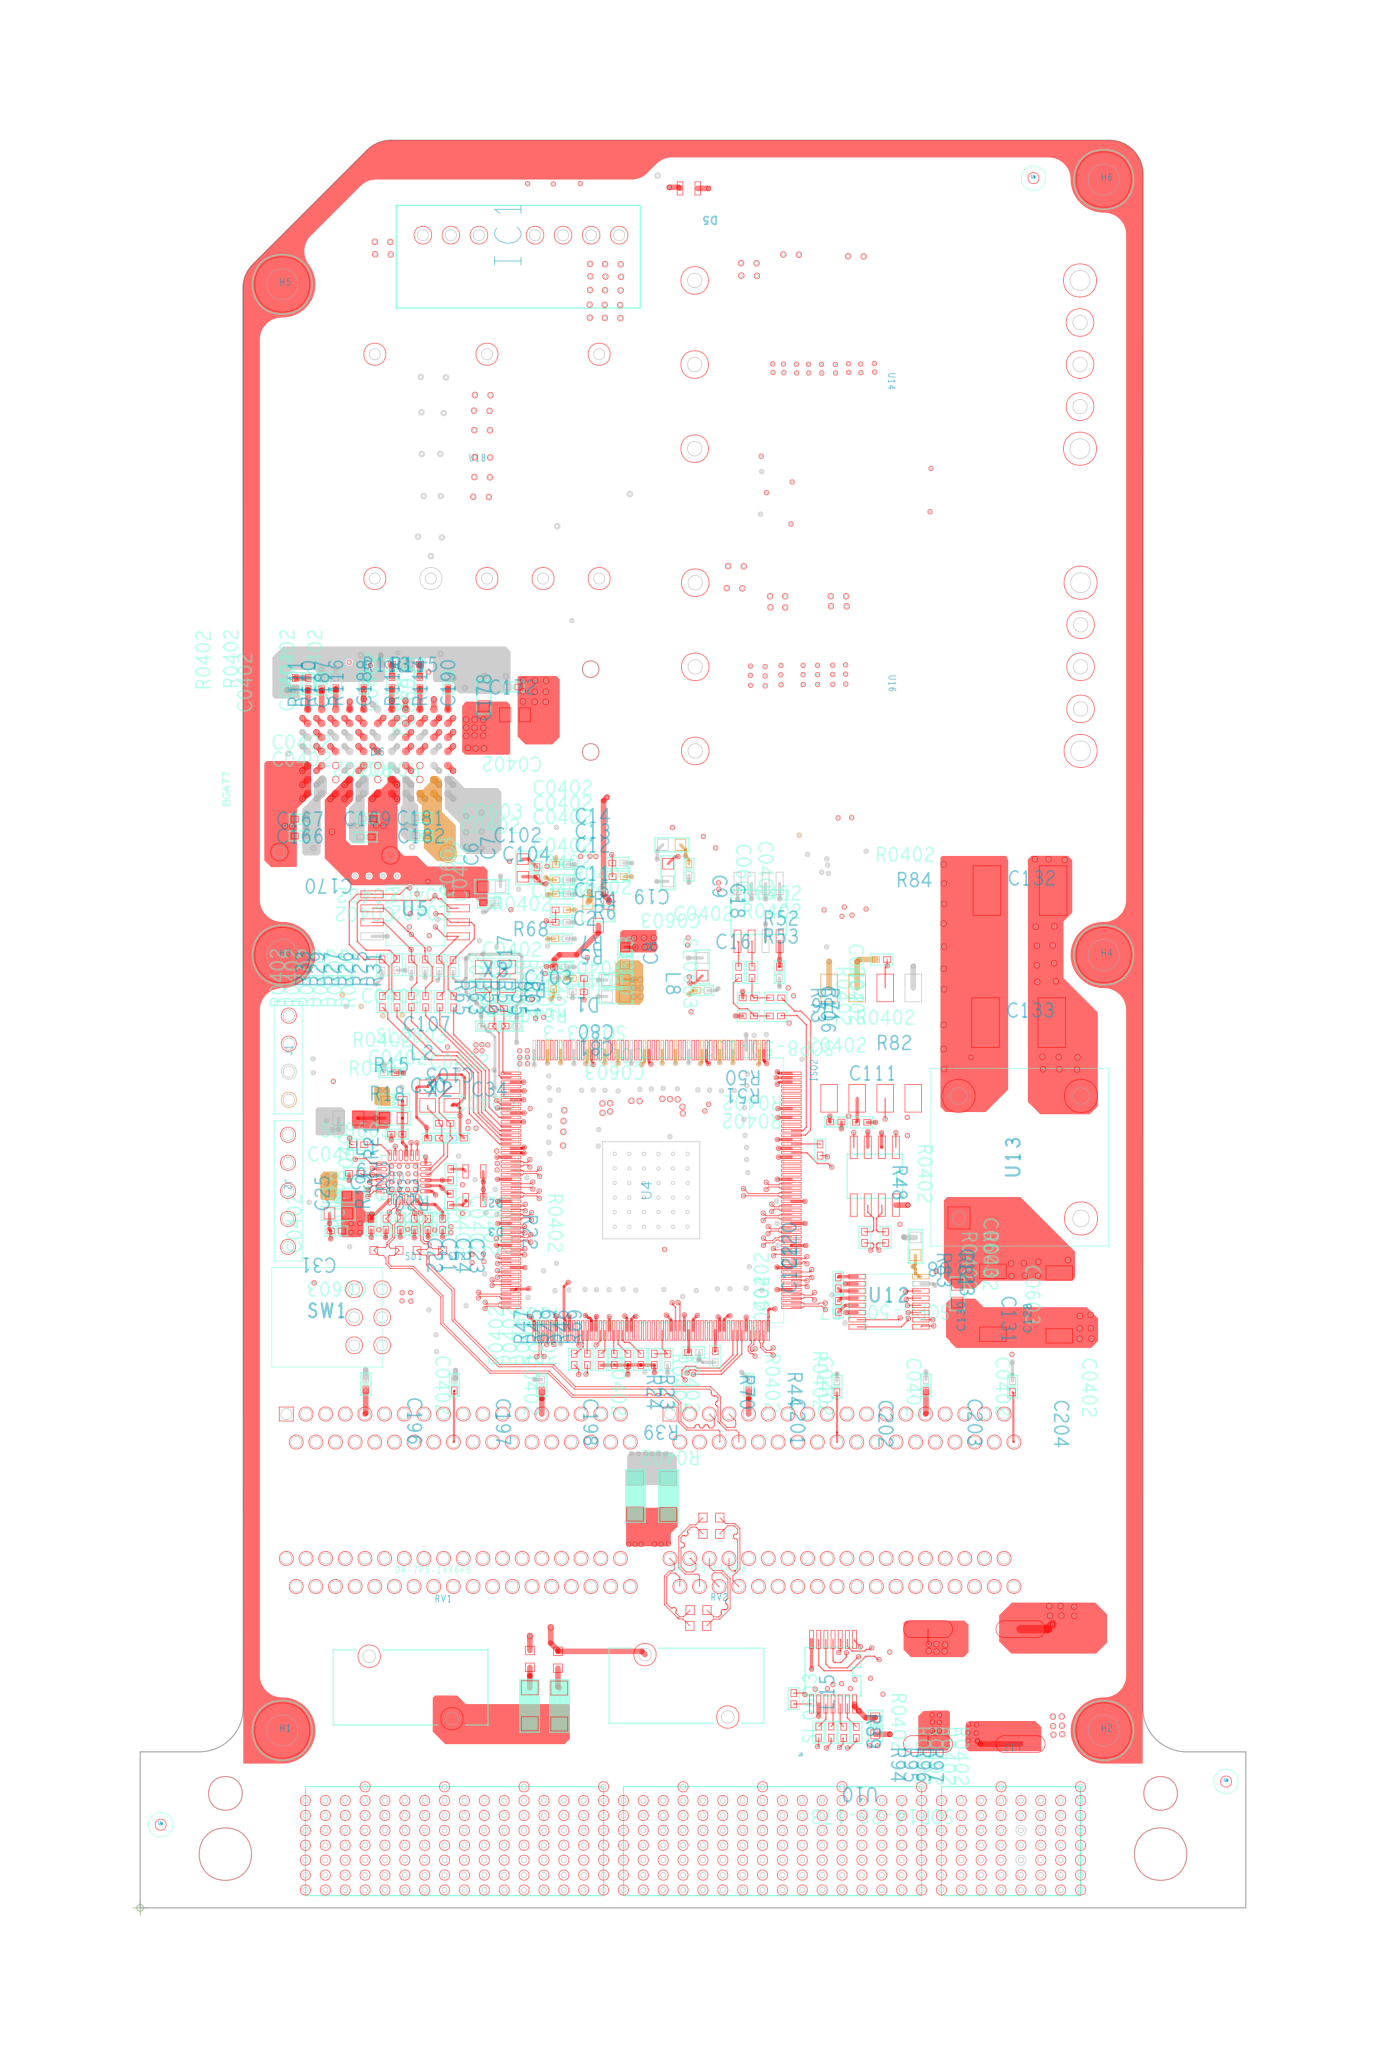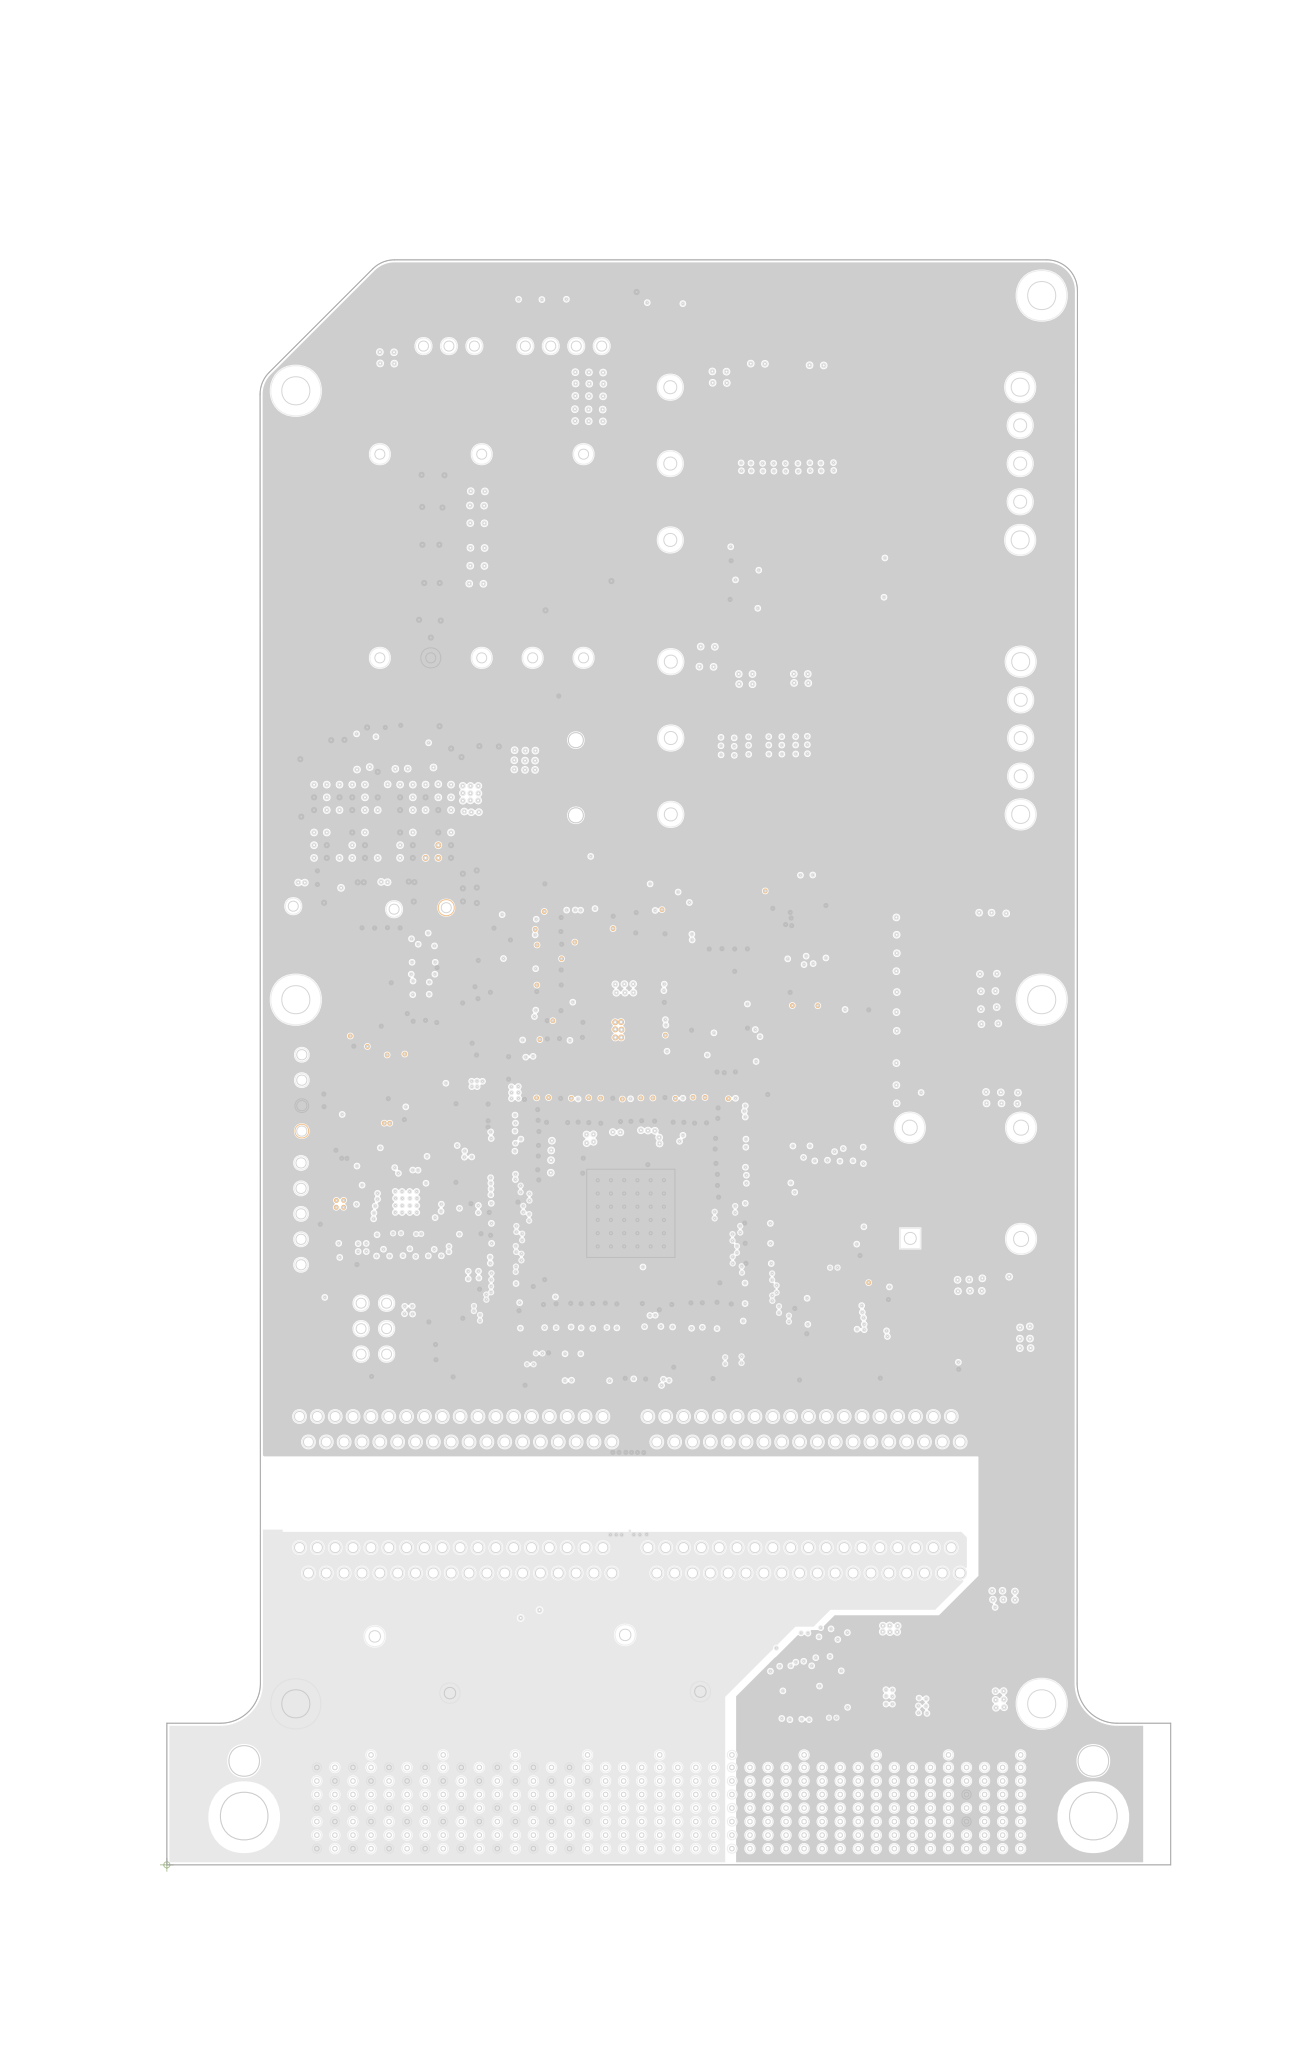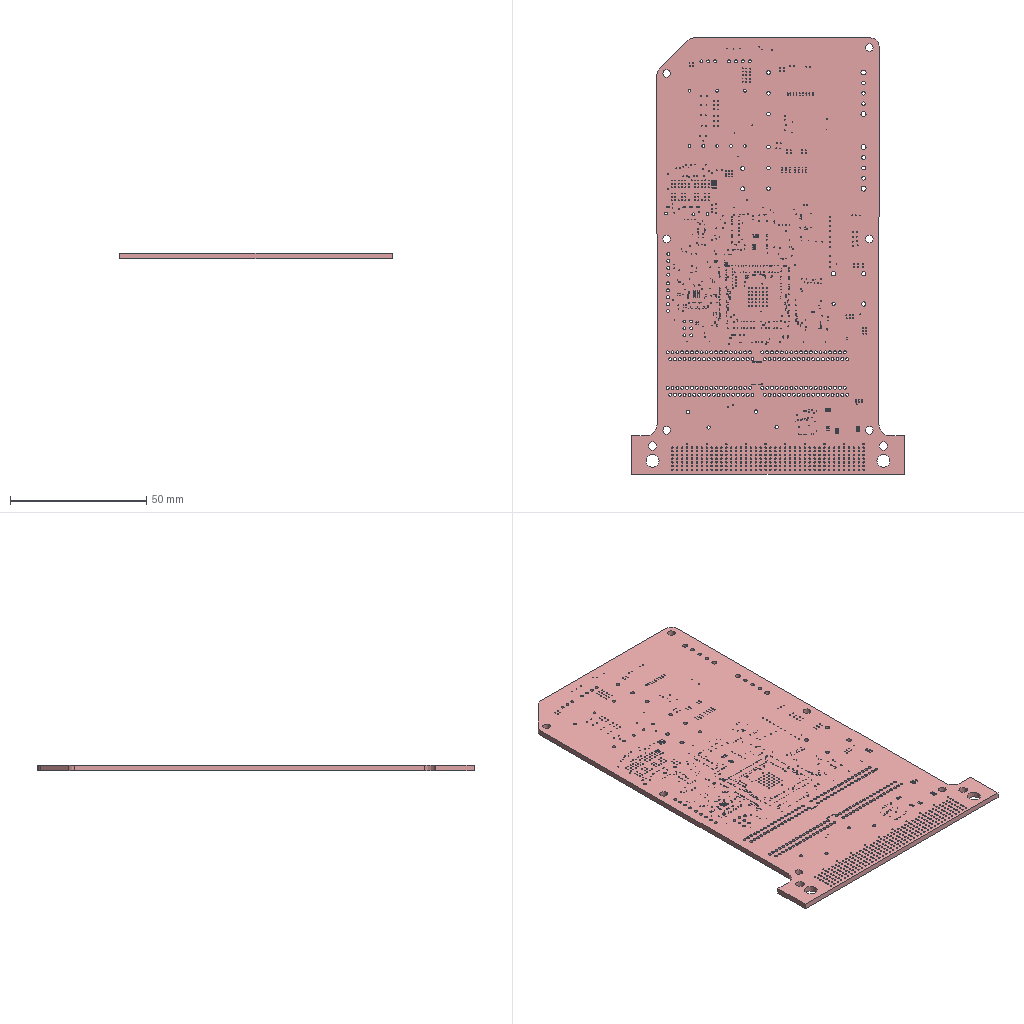Circuit board layout | Cadence Allegro | box 100.1 x 160.1 x 2.1 mm
Layer stack:
# Cadence Allegro layer stack of  (unit mm; from the constraint file cross-section; dielectric type: 0 not recorded (Allegro does not mark core vs prepreg), 3 surface material)
index,name,kind,layer,copper_thickness_mm,dielectric_type,dielectric_thickness_mm,dielectric_material,dielectric_constant
0,Top Surface,other,,,,,,
1,TOP,copper,TOP,0.0305,,,,
2,Dielectric1,dielectric,,,0,0.2032,FR-4,4.5
3,GND2,copper,GND2,0.0305,,,,
4,Dielectric2,dielectric,,,0,0.2032,FR-4,4.5
5,SIG3,copper,SIG3,0.0305,,,,
6,Dielectric3,dielectric,,,0,0.2032,FR-4,4.5
7,POWER4,copper,POWER4,0.0305,,,,
8,Dielectric4,dielectric,,,0,0.2032,FR-4,4.5
9,POWER5,copper,POWER5,0.0305,,,,
10,Dielectric5,dielectric,,,0,0.2032,FR-4,4.5
11,POWER6,copper,POWER6,0.0305,,,,
12,Dielectric6,dielectric,,,0,0.2032,FR-4,4.5
13,GND7,copper,GND7,0.0305,,,,
14,Dielectric7,dielectric,,,0,0.2032,FR-4,4.5
15,SIG8,copper,SIG8,0.0305,,,,
16,Dielectric8,dielectric,,,0,0.2032,FR-4,4.5
17,GND9,copper,GND9,0.0305,,,,
18,Dielectric9,dielectric,,,0,0.2032,FR-4,4.5
19,BOTTOM,copper,BOTTOM,0.0305,,,,
20,Bottom Surface,other,,,,,,
# drill layer pairs: low layer,high layer
drill_pair,TOP,BOTTOM
Part placement:
REFDES,COMP_VALUE,SYM_NAME,SYM_X,SYM_Y,SYM_ROTATE,SYM_MIRROR
BT1,CR1220,CR1220,1606.230,4275.930,270.000,YES
C1,2pF,SC0402,1221.830,3337.342,90.000,YES
C2,0.1uF/16V,SC0402,1496.000,3355.000,0.000,NO
C3,2pF,SC0402,1222.830,3247.342,270.000,YES
C4,20pF,SC0402,1246.470,3532.310,270.000,YES
C5,20pF,SC0402,1246.470,3447.310,90.000,YES
C6,1uF/50V,SC0603,1364.028,3708.722,90.000,NO
C7,0.1uF/16V,SC0402,1414.460,3690.992,90.000,NO
C8,2.2uF,SC0603,2004.278,3356.092,90.000,NO
C9,2.2uF,SC0603,1882.000,3692.000,270.000,NO
C10,0.1uF/16V,SC0402,663.890,2861.622,270.000,YES
C11,0.1uF/16V,SC0402,1501.000,3515.000,0.000,NO
C12,0.1uF/16V,SC0402,1502.000,3616.000,0.000,NO
C13,0.1uF/16V,SC0402,1502.000,3666.000,0.000,NO
C14,0.1uF/16V,SC0402,1502.000,3721.000,0.000,NO
C15,0.1uF/16V,SC0402,1499.000,3456.000,0.000,NO
C16,0.1uF/16V,SC0402,2003.884,3271.776,0.000,NO
C17,0.1uF/16V,SC0402,1474.000,3296.000,90.000,NO
C18,0.1uF/16V,SC0402,1956.210,3702.418,270.000,NO
C19,10uF/6.3V,SC0603,1895.000,3791.000,180.000,NO
C20,0.1uF/16V,SC0402,757.158,3235.510,90.000,YES
C21,10pF/16V,SC0402,927.190,2437.606,270.000,NO
C22,10pF/16V,SC0402,876.098,2438.000,270.000,NO
C23,10pF/16V,SC0402,1025.920,2437.424,270.000,NO
C24,10pF/16V,SC0402,977.252,2437.818,270.000,NO
C25,0.1uF/16V,SC0402,823.460,2437.284,90.000,NO
C26,0.1uF/16V,SC0402,1022.720,2735.994,90.000,YES
C27,0.1uF/16V,SC0402,1061.720,2735.994,90.000,YES
C28,0.1uF/16V,SC0402,1128.810,2502.688,0.000,YES
C29,10uF/6.3V,SC0603,903.442,2816.312,180.000,NO
C30,0.1uF/16V,SC0402,914.868,2758.788,0.000,NO
C31,10uF/6.3V,SC0603,706.442,2476.684,180.000,NO
C32,0.1uF/16V,SC0402,698.956,2414.038,0.000,NO
C33,20pF,SC0402,1046.034,2745.002,180.000,NO
C34,20pF,SC0402,1134.034,2745.002,0.000,NO
C35,10uF/6.3V,SC0603,1122.900,2178.426,90.000,YES
C36,0.1uF/16V,SC0402,2240.284,2157.150,270.000,YES
C37,0.1uF/16V,SC0402,2224.918,2285.988,0.000,YES
C38,0.1uF/16V,SC0402,2215.068,2622.464,0.000,YES
C39,0.1uF/16V,SC0402,1531.000,2158.000,270.000,YES
C40,0.1uF/16V,SC0402,2326.176,2441.224,0.000,YES
C41,0.1uF/16V,SC0402,1323.446,2603.158,180.000,YES
C42,0.1uF/16V,SC0402,1303.352,2455.408,270.000,YES
C43,0.1uF/16V,SC0402,1418.794,2294.656,180.000,YES
C44,0.1uF/16V,SC0402,1407.762,2156.362,270.000,YES
C45,0.1uF/16V,SC0402,2160.302,2161.484,270.000,YES
C46,0.1uF/16V,SC0402,1214.308,2620.888,0.000,YES
C47,0.1uF/16V,SC0402,2323.812,2520.812,0.000,YES
C48,0.1uF/16V,SC0402,2213.886,2667.380,0.000,YES
C49,0.1uF/16V,SC0402,2226.100,2234.374,0.000,YES
C50,10uF/6.3V,SC0603,1203.276,2680.776,0.000,YES
C51,0.1uF/16V,SC0402,1304.140,2542.482,270.000,YES
C52,0.1uF/16V,SC0402,1418.794,2231.222,180.000,YES
C53,0.1uF/16V,SC0402,1479.000,2157.000,270.000,YES
C54,10uF/6.3V,SC0603,1279.712,2956.182,0.000,YES
C55,0.1uF/16V,SC0402,1412.884,2825.768,180.000,YES
C56,0.1uF/16V,SC0402,2210.272,2973.000,0.000,YES
C57,0.1uF/16V,SC0402,2212.060,2811.420,0.000,YES
C58,0.1uF/16V,SC0402,2053.528,2160.302,270.000,YES
C59,0.1uF/16V,SC0402,1721.698,2158.000,270.000,YES
C60,0.1uF/16V,SC0402,1415.758,2924.426,180.000,YES
C61,0.1uF/16V,SC0402,1412.096,2690.232,180.000,YES
C62,0.1uF/16V,SC0402,2213.576,2712.088,0.000,YES
C63,0.1uF/16V,SC0402,1955.028,2160.302,270.000,YES
C64,0.1uF/16V,SC0402,1627.000,2158.000,270.000,YES
C65,10uF/6.3V,SC0603,1574.196,2775.534,180.000,YES
C66,10uF/6.3V,SC0603,1573.242,2716.630,180.000,YES
C67,0.1uF/16V,SC0402,1672.000,2159.000,270.000,YES
C68,0.1uF/16V,SC0402,2003.490,2160.302,270.000,YES
C69,0.1uF/16V,SC0402,2102.778,2160.696,270.000,YES
C70,0.1uF/16V,SC0402,2211.576,2755.088,0.000,YES
C71,0.1uF/16V,SC0402,2211.060,2853.420,0.000,YES
C72,0.1uF/16V,SC0402,1412.490,2730.026,180.000,YES
C73,0.1uF/16V,SC0402,1414.758,2966.426,180.000,YES
C74,0.1uF/16V,SC0402,1415.758,2880.426,180.000,YES
C75,0.1uF/16V,SC0402,2211.272,2932.000,0.000,YES
C76,0.1uF/16V,SC0402,1586.000,2158.000,270.000,YES
C77,0.1uF/16V,SC0402,1412.096,2784.004,180.000,YES
C78,0.1uF/16V,SC0402,1867.166,2156.756,270.000,YES
C79,0.1uF/16V,SC0402,1762.362,2157.544,270.000,YES
C80,10uF/6.3V,SC0603,1695.382,3309.206,180.000,NO
C81,10uF/6.3V,SC0603,1695.776,3250.106,180.000,NO
C82,0.1uF/16V,SC0402,1988.274,2963.728,90.000,YES
C83,0.1uF/16V,SC0402,1657.000,2959.000,90.000,YES
C84,0.1uF/16V,SC0402,2189.064,3056.258,270.000,YES
C85,0.1uF/16V,SC0402,1864.486,2963.910,90.000,YES
C86,0.1uF/16V,SC0402,1781.486,2962.910,90.000,YES
C87,0.1uF/16V,SC0402,1915.486,2962.910,90.000,YES
C88,0.1uF/16V,SC0402,1574.000,2958.000,90.000,YES
C89,0.1uF/16V,SC0402,1435.342,3034.982,0.000,YES
C90,0.1uF/16V,SC0402,1491.000,2962.000,90.000,YES
C91,0.1uF/16V,SC0402,1704.000,2959.000,90.000,YES
C92,0.1uF/16V,SC0402,2119.274,2962.728,90.000,YES
C93,0.1uF/16V,SC0402,2072.274,2962.728,90.000,YES
C94,0.1uF/16V,SC0402,1822.486,2963.910,90.000,YES
C95,0.1uF/16V,SC0402,2030.274,2963.728,90.000,YES
C96,0.1uF/16V,SC0402,1615.000,2959.000,90.000,YES
C97,10uF/6.3V,SC0603,1233.614,2407.734,270.000,YES
C98,0.1uF/16V,SC0402,2232.798,3056.258,270.000,YES
C99,0.1uF/16V,SC0402,1249.768,2304.506,90.000,YES
C100,0.1uF/16V,SC0402,2324.600,2362.030,0.000,YES
C101,10uF/6.3V,SC0603,1888.836,2812.372,90.000,YES
C102,1uF/50V,SC0603,1253.116,3641.850,0.000,NO
C103,27pF,SC0402,1322.084,3144.390,0.000,NO
C104,0.1uF/16V,SC0402,1244.116,3583.850,0.000,NO
C105,27pF,SC0402,1236.084,3144.390,180.000,NO
C106,0.1uF/16V,SC0402,2278.896,3336.392,270.000,NO
C107,0.1uF/16V,SC0402,889.652,2978.246,0.000,NO
C108,0.1uF/16V,SC0402,702.502,2357.696,180.000,YES
C109,0.1uF/16V,SC0402,1115.414,2956.576,180.000,YES
C110,100pF,SC0402,668.618,2977.852,0.000,YES
C111,0.1uF/16V,SC0402,2480.230,2802.522,0.000,NO
C112,0.1uF/16V,SC0402,2623.252,2730.420,180.000,YES
C113,0.1uF/16V,SC0402,2470.380,3406.918,270.000,YES
C114,0.1uF/16V,SC0402,2379.630,3805.304,270.000,YES
C115,0.1uF/16V,SC0402,2460.136,3536.150,180.000,YES
C116,10uF/6.3V,SC0603,2609.462,730.476,270.000,YES
C117,0.1uF/16V,SC0402,2535.390,735.204,270.000,YES
C118,0.1uF/16V,SC0402,2406.552,733.628,270.000,YES
C119,0.1uF/16V,SC0402,2767.456,2240.284,270.000,YES
C120,0.1uF/16V,SC0402,2488.898,2228.858,90.000,NO
C121,0.1uF/16V,SC0402,2488.898,2205.612,270.000,YES
C122,0.1uF/16V,SC0402,2489.292,2144.148,90.000,NO
C123,10uF/6.3V,SC0603,2763.910,2359.272,270.000,NO
C124,0.1uF/16V,SC0402,2490.868,2105.930,90.000,YES
C125,22uF/50V,SC7343,2951.000,897.000,90.000,YES
C126,JCT41V-1812-X7R-1KV-472K,SC1812,3309.000,903.000,90.000,YES
C127,22uF/50V,SC7343,2749.000,895.000,90.000,YES
C128,22uF/50V,SC7343,3277.000,2152.000,90.000,NO
C129,JCT41V-1812-X7R-1KV-472K,SC1812,2799.000,660.000,0.000,YES
C130,22uF/50V,SC7343,3040.498,2157.938,90.000,NO
C131,1uF/50V,SC0603,2912.842,2190.246,270.000,NO
C132,22uF/50V,CAP_CASE_D,3137.090,3628.000,0.000,NO
C133,22uF/50V,CAP_CASE_D,3132.090,3157.000,0.000,NO
C134,22uF/50V,CAP_CASE_D,1408.939,5767.372,180.000,YES
C135,22uF/50V,CAP_CASE_D,990.915,5767.372,0.000,YES
C136,10uF/50V,SC0805,1047.646,6108.182,0.000,YES
C137,10uF/50V,SC0805,1607.126,6109.364,270.000,YES
C138,10uF/50V,SC0805,1516.506,6108.182,270.000,YES
C139,10uF/50V,SC0805,1428.250,6108.970,270.000,YES
C140,22uF/50V,CAP_CASE_D,2546.816,5697.240,270.000,YES
C141,22uF/50V,CAP_CASE_D,2324.994,5694.088,270.000,YES
C142,JCT41V-1812-X7R-1KV-472K,SC1812,3381.000,5038.000,0.000,YES
C143,1uF/50V,SC0603,2167.788,5727.972,270.000,YES
C144,47uF/25V,CAP_CASE_D,2812.000,5522.900,270.000,YES
C145,47uF/25V,CAP_CASE_D,3040.000,5523.910,270.000,YES
C146,0.1uF/16V,SC0603,2292.836,5122.312,0.000,YES
C147,JCT41V-1812-X7R-1KV-472K,SC1812,3200.000,6039.000,270.000,YES
C148,JCT41V-1812-X7R-1KV-472K,SC1812,3358.000,3945.000,0.000,YES
C149,22uF/50V,CAP_CASE_D,2497.960,4623.590,270.000,YES
C150,22uF/50V,CAP_CASE_D,2278.502,4623.590,270.000,YES
C151,1uF/50V,SC0603,2112.628,4604.284,270.000,YES
C152,47uF/25V,CAP_CASE_D,3048.000,4443.900,270.000,YES
C153,47uF/25V,CAP_CASE_D,2832.000,4445.910,270.000,YES
C154,0.1uF/16V,SC0603,2289.112,4970.312,0.000,YES
C155,JCT41V-1812-X7R-1KV-472K,SC1812,3383.000,4881.000,180.000,YES
C156,JCT41V-1812-X7R-1KV-472K,SC1812,604.396,5241.382,180.000,YES
C157,22uF/50V,CAP_CASE_D,1445.552,5090.862,0.000,YES
C158,22uF/50V,CAP_CASE_D,1451.542,5327.862,0.000,YES
C159,1uF/50V,SC0603,1442.452,5481.862,0.000,YES
C160,JCT41V-1812-X7R-1KV-472K,SC1812,966.876,5413.560,0.000,YES
C161,47uF/10V,CASE-C-6032,832.916,4956.914,180.000,YES
C162,47uF/10V,CASE-C-6032,831.734,5255.172,180.000,YES
C163,47uF/10V,CASE-C-6032,832.916,5110.574,180.000,YES
C164,47uF/6.3V,SC0805,582.206,3898.026,180.000,YES
C165,47uF/6.3V,SC0805,582.206,3819.026,180.000,YES
C166,0.1uF/16V,SC0402,571.300,3822.588,0.000,NO
C167,1000pF/25V,SC0402,571.300,3882.870,0.000,NO
C168,47uF/6.3V,SC0805,802.998,3899.058,0.000,YES
C169,0.1uF/16V,SC0402,811.246,3884.840,180.000,NO
C170,1000pF/25V,SC0402,804.548,3819.042,180.000,NO
C171,22uF/6.3V,SC0805,942.448,4839.502,180.000,YES
C172,0.1uF/16V,SC0402,1328.962,4354.094,180.000,NO
C173,22uF/6.3V,SC0805,756.874,4099.964,0.000,YES
C174,22uF/6.3V,SC0805,1054.344,4100.752,0.000,YES
C175,47uF/6.3V,SC0805,802.998,3820.058,0.000,YES
C176,22uF/6.3V,SC0805,906.594,4099.964,0.000,YES
C177,22uF/6.3V,SC0805,607.154,4101.146,0.000,YES
C178,1uF/50V,SC0603,1224.946,4317.846,90.000,NO
C179,47uF/6.3V,SC0805,1005.512,3899.694,0.000,YES
C180,47uF/6.3V,SC0805,1005.512,3823.694,0.000,YES
C181,0.1uF/16V,SC0402,999.578,3887.204,180.000,NO
C182,1000pF/25V,SC0402,1002.730,3823.770,180.000,NO
C183,0.1uF/16V,SC0402,674.922,4171.672,0.000,YES
C184,0.1uF/16V,SC0402,822.672,4221.316,0.000,YES
C185,0.1uF/16V,SC0402,941.266,4196.100,270.000,YES
C186,0.1uF/16V,SC0402,1061.042,4219.740,180.000,YES
C187,10pF/16V,SC0402,646.948,4365.520,90.000,NO
C188,10pF/16V,SC0402,797.456,4369.460,90.000,NO
C189,10nF/16V,SC0402,596.910,4200.040,270.000,YES
C190,10pF/16V,SC0402,1096.896,4369.066,90.000,NO
C191,10nF/16V,SC0402,748.600,4199.646,270.000,YES
C192,10nF/16V,SC0402,1063.012,4280.416,180.000,YES
C193,4.7uF/16V,SC0805,1068.922,4395.070,270.000,YES
C194,4.7uF/16V,SC0805,641.432,4340.698,0.000,YES
C195,4.7uF/16V,SC0805,918.414,4389.948,270.000,YES
C196,0.1uF/16V,SC0402,804.000,1868.000,270.000,NO
C197,0.1uF/16V,SC0402,1120.142,1864.802,270.000,NO
C198,0.1uF/16V,SC0402,1431.796,1864.014,270.000,NO
C199,0.1uF/16V,SC0402,1774.182,1892.776,90.000,YES
C200,1nF/2KV,SC1206,1389.072,720.672,270.000,NO
C201,0.1uF/16V,SC0402,2169.758,1864.802,270.000,NO
C202,0.1uF/16V,SC0402,2484.170,1858.892,270.000,NO
C203,0.1uF/16V,SC0402,2801.734,1863.620,270.000,NO
C204,0.1uF/16V,SC0402,3110.630,1858.892,270.000,NO
C205,1nF/2KV,SC1206,1494.072,719.682,270.000,NO
C206,1nF/2KV,SC1206,1882.925,1467.059,270.000,NO
C207,1nF/2KV,SC1206,1764.331,1468.241,270.000,NO
D1,BAT54C,SOT23-3,1633.524,3545.212,180.000,NO
D2,LED-G,SD0805,1191.456,2626.404,180.000,NO
D3,LED-Y,SD0805,1191.850,2523.964,180.000,NO
D4,TVS/P6KE39A,DO-214AC,3133.210,903.560,270.000,YES
D5,LED-R,SD0805,1956.210,6132.216,180.000,NO
D6,LTM4644IY,BGA77-1R27-15X9,847.000,4124.000,90.000,NO
F1,3A/50V,F1206,3121.020,666.610,0.000,YES
H1,SCREW-D7-d3p2,SCREW-D6-D3P2,506.430,632.470,0.000,NO
H2,SCREW-D7-d3p2,SCREW-D6-D3P2,3435.570,632.420,0.000,NO
H3,SCREW-D7-d3p2,SCREW-D6-D3P2,506.430,3398.170,0.000,NO
H4,SCREW-D7-d3p2,SCREW-D6-D3P2,3435.580,3398.170,0.000,NO
H5,SCREW-D7-d3p2,SCREW-D6-D3P2,506.430,5789.900,0.000,NO
H6,SCREW-D7-d3p2,SCREW-D6-D3P2,3435.570,6163.920,0.000,NO
IC1,VRB2403S-10WR3,VRB24XXS,1357.714,5965.494,90.000,NO
ISO1,6N173,DIP8,2409.508,3225.970,180.000,YES
ISO2,6N173,DIP8,2413.789,2946.048,0.000,NO
J1,CON4,SIP_254_4P,529.970,2882.000,90.000,NO
J2,DBUG_PPU,SIP_254_5P,527.030,2757.000,270.000,NO
J3,jvpx-21t8aac8-b,JVPX-21T8AAC8-B,3352.900,63.570,0.000,NO
L1,1A,SL0603,707.624,2540.118,0.000,NO
L2,1A,SL0603,905.412,2878.170,0.000,NO
L3,3A,SL0805,742.296,2816.312,0.000,NO
L4,1A,SL0603,1036.220,2213.886,180.000,YES
L5,1A,SL0603,1234.796,2768.244,90.000,YES
L6,3A,SL0805,1282.864,3034.588,180.000,YES
L7,1A,SL0603,1577.576,2836.800,0.000,YES
L8,1A,SL0603,1728.478,3395.492,270.000,NO
L9,1A,SL0603,1793.882,2844.680,180.000,YES
L10,1A,SL0603,1144.176,2378.184,180.000,YES
L11,1A,SL0603,641.432,2486.140,270.000,YES
L12,JSMT121205-610/610,PA2744,3139.000,584.080,180.000,NO
L13,5A,SL0805,1336.448,4254.806,180.000,NO
L14,1A,SL0603,2735.148,2317.508,180.000,YES
L15,1A,SL0603,2620.888,648.918,90.000,NO
R1,1M 1%,SR0402,1272.830,3292.342,90.000,YES
R2,1M 1%,SR0402,1298.470,3485.310,270.000,YES
R3,10K 1%,SR0402,1501.000,3559.000,180.000,NO
R4,5.1K/NC,SR0402,1562.210,3314.328,0.000,NO
R5,5.1K,SR0402,1704.050,3677.596,180.000,NO
R6,5.1K,SR0402,1561.816,3266.654,0.000,NO
R7,5.1K/NC,SR0402,1703.262,3726.058,180.000,NO
R8,2.2K,SR0402,865.158,3232.510,90.000,YES
R9,2.2K,SR0402,931.022,3233.164,90.000,YES
R10,10K 1%,SR0402,811.158,3234.510,90.000,YES
R11,49R9 1%,SR0402,927.190,2438.606,270.000,YES
R12,49R9 1%,SR0402,876.098,2438.000,270.000,YES
R13,49R9 1%,SR0402,1025.920,2437.424,270.000,YES
R14,49R9 1%,SR0402,977.252,2438.818,270.000,YES
R15,33 1%,SR0402,778.938,2721.752,0.000,NO
R16,10K 1%,SR0402,1129.598,2605.522,180.000,YES
R17,10K 1%,SR0402,1129.204,2554.696,180.000,YES
R18,10K 1%,SR0402,764.754,2619.706,0.000,NO
R19,12.1K,SR0402,1077.984,2437.678,90.000,NO
R20,1M 1%,SR0402,1085.470,2797.794,180.000,NO
R21,330R 1%,SR0402,1107.140,2614.584,90.000,NO
R22,330R 1%,SR0402,1105.958,2526.722,270.000,NO
R23,0 1%,SR0402,1594.518,1956.210,270.000,NO
R24,0 1%,SR0402,1547.632,1956.210,270.000,NO
R25,0 1%,SR0402,1068.134,3231.982,90.000,NO
R26,0 1%,SR0402,1017.308,3231.588,90.000,NO
R27,0 1%,SR0402,966.876,3231.982,90.000,NO
R28,1K 1%,SR0402,1009.034,2107.900,0.000,YES
R29,0 1%,SR0402,915.656,3231.588,90.000,NO
R30,1K 1%,SR0402,1009.428,2043.678,0.000,YES
R31,0 1%,SR0402,1117.384,3231.194,90.000,NO
R32,1K 1%,SR0402,1010.610,1983.790,0.000,YES
R33,0 1%,SR0402,863.648,3231.982,90.000,NO
R34,0 1%,SR0402,2314.908,2955.206,270.000,YES
R35,4.7K 1%,SR0402,1891.200,2328.146,90.000,YES
R36,33 1%,SR0402,1890.806,2243.830,90.000,YES
R37,4.7K 1%,SR0402,1936.904,2327.752,90.000,YES
R38,33 1%,SR0402,1937.298,2243.436,90.000,YES
R39,1K 1%,SR0402,1973.546,1980.638,180.000,NO
R40,2.1K 1%,SR0402,1525.174,2315.932,180.000,YES
R41,390R 1%,SR0402,1525.568,2261.560,0.000,YES
R42,4.7K 1%,SR0402,1319.790,2895.728,0.000,YES
R43,4.7K 1%,SR0402,1318.790,2847.728,0.000,YES
R44,1K 1%,SR0402,2050.376,1965.272,270.000,NO
R45,4.7K 1%,SR0402,1690.654,1955.422,90.000,NO
R46,4.7K 1%,SR0402,1785.214,1955.816,90.000,NO
R47,4.7K 1%,SR0402,1643.374,1955.422,90.000,NO
R48,33 1%,SR0402,2424.282,2702.840,270.000,NO
R49,4.7K 1%,SR0402,1738.570,1955.854,90.000,NO
R50,33 1%,SR0402,2266.096,3245.542,180.000,NO
R51,33 1%,SR0402,2264.712,3180.762,180.000,NO
R52,4.7K 1%,SR0402,2168.338,3245.116,0.000,NO
R53,4.7K 1%,SR0402,2167.792,3180.842,0.000,NO
R54,4.7K 1%,SR0402,1007.064,3498.326,180.000,YES
R55,1K 1%,SR0402,1065.770,3361.214,270.000,NO
R56,4.7K 1%,SR0402,1010.610,3445.136,0.000,YES
R57,1K 1%,SR0402,1015.732,3362.396,270.000,NO
R58,4.7K 1%,SR0402,1010.216,3395.492,0.000,YES
R59,1K 1%,SR0402,967.270,3363.184,270.000,NO
R60,4.7K 1%,SR0402,1007.064,3545.212,180.000,YES
R61,1K 1%,SR0402,1115.414,3360.426,270.000,NO
R62,4.7K 1%,SR0402,1007.064,3593.280,180.000,YES
R63,1K 1%,SR0402,914.474,3363.578,270.000,NO
R64,4.7K 1%,SR0402,1006.276,3638.984,0.000,YES
R65,1K 1%,SR0402,862.466,3362.396,270.000,NO
R66,4.7K 1%,SR0402,2313.962,3101.568,90.000,YES
R67,1K 1%,SR0402,2332.874,3025.920,180.000,YES
R68,1M 1%,SR0402,1276.720,3206.806,0.000,NO
R69,4.7K 1%,SR0402,1833.264,1955.718,90.000,NO
R70,1K 1%,SR0402,1880.264,1955.718,270.000,NO
R71,0 1%,SR0402,2181.366,3336.264,270.000,NO
R72,0 1%,SR0402,1112.262,3012.524,0.000,YES
R73,0 1%,SR0402,2133.366,3336.264,270.000,NO
R74,0 1%,SR0402,1096.108,2839.952,270.000,YES
R75,4.7K 1%,SR0402,1115.414,2905.750,0.000,YES
R76,1K 1%,SR0402,669.012,3027.496,0.000,YES
R77,330R 1%,SR0402,2626.404,3407.706,90.000,YES
R78,4.7K 1%,SR0402,2715.448,2730.420,0.000,YES
R79,5R1,SR0402,2523.964,3406.918,90.000,YES
R80,120R,SR0603,2611.826,625.278,0.000,YES
R81,5R1,SR0402,2657.924,2391.186,270.000,NO
R82,5R1,SR0402,2572.426,2801.340,0.000,NO
R83,5R1,SR0402,2582.670,2391.186,270.000,NO
R84,4.7K 1%,SR0402,2643.346,3382.096,0.000,NO
R85,0 1%,SR0402,2709.144,2484.564,270.000,YES
R86,330R 1%,SR0402,2521.206,2730.420,180.000,YES
R87,4.7K 1%,SR0402,2611.826,949.146,0.000,YES
R88,330R 1%,SR0402,2469.986,841.584,90.000,YES
R89,0 1%,SR0402,2330.116,745.842,270.000,NO
R90,330R 1%,SR0402,2521.994,840.402,90.000,YES
R91,330R 1%,SR0402,2574.002,840.008,90.000,YES
R92,10K 1%,SR0402,2450.286,732.446,90.000,YES
R93,330R 1%,SR0402,2627.192,839.614,90.000,YES
R94,330R 1%,SR0402,2418.766,626.460,270.000,NO
R95,330R 1%,SR0402,2463.682,626.460,270.000,NO
R96,330R 1%,SR0402,2508.204,625.672,270.000,NO
R97,330R 1%,SR0402,2553.514,625.278,270.000,NO
R98,1K 1%,SR0603,1733.206,6114.880,180.000,YES
R99,4.7K 1%,SR0603,2167.788,5550.278,90.000,YES
R100,NC,SR0603,3183.914,5457.688,270.000,YES
R101,5R1,SR0603,2771.836,5163.312,90.000,YES
R102,NC,SR0603,3184.702,5599.528,270.000,YES
R103,510R,SR0603,2290.836,5185.312,180.000,YES
R104,5R1,SR0603,2771.396,5008.922,90.000,YES
R105,4.7K 1%,SR0603,2109.870,4316.664,0.000,YES
R106,NC,SR0603,3197.310,4367.490,270.000,YES
R107,NC,SR0603,3198.098,4500.662,270.000,YES
R108,510R,SR0603,2291.112,5043.312,180.000,YES
R109,4.7K 1%,SR0603,1627.452,4893.862,90.000,YES
R110,0 1%,SR0402,598.664,4365.812,90.000,NO
R111,60.4K 1%,SR0402,552.782,4366.308,270.000,NO
R112,350R 1%,SR0402,897.532,4369.460,90.000,NO
R113,6.3K 1%,SR0402,877.044,4435.258,180.000,NO
R114,3.3K 1%,SR0402,996.820,4369.460,90.000,NO
R115,10K 1%,SR0402,977.908,4434.864,180.000,NO
R116,10K 1%,SR0402,697.380,4369.460,90.000,NO
R117,10K 1%,SR0603,994.062,4377.340,90.000,YES
R118,10K 1%,SR0603,745.054,4375.764,90.000,YES
R119,1K 1%,SR0603,849.070,4373.400,90.000,YES
R120,75 1%,SR0603,1389.472,887.662,270.000,NO
R121,75 1%,SR0603,1489.472,884.662,270.000,NO
R122,0 1%,SR0603,1989.700,1005.488,0.000,NO
R123,0 1%,SR0603,1990.882,1061.830,0.000,NO
R124,0 1%,SR0603,2036.586,1333.690,0.000,NO
R125,0 1%,SR0603,2036.586,1391.608,0.000,NO
RV1,FNR-10K471,DR2-7P5-14X6P8,964.113,785.884,0.000,NO
RV2,FNR-10K471,DR2-7P5-14X6P8,1947.537,791.794,0.000,NO
SD1,ESD03V32D-LCD,D-SOD323,878.226,2344.694,0.000,NO
SD2,ESD03V32D-LCD,D-SOD323,1032.280,2344.300,0.000,NO
SW1,NDA-03V,SWD6-100-10X9-R,666.000,2106.000,0.000,NO
T1,UTG72T13B,TFMD72-0418-1935,521.000,1761.000,180.000,YES
T2,UTG72T13B,TFMD72-0418-1935,1889.000,1761.000,180.000,YES
TP1,test_cir,TP-PWR,496.440,3765.458,0.000,YES
TP2,test_cir,TP-PWR,892.410,3753.638,0.000,YES
TP3,test_cir,TP-PWR,1097.290,3759.548,0.000,YES
U1,xxxxx,LQFP-100,1701.000,3495.000,270.000,YES
U2,CAT24C256W,SOIC-8-751BE,841.158,3479.510,180.000,YES
U3,xy,QFN24,938.902,2604.734,180.000,NO
U4,xx,QFP216-040-24X24-T-SQ8P8,1822.000,2559.000,90.000,NO
U5,xxx,SOP8-50-210,980.272,3539.696,0.000,NO
U6,AT24C64D-SSHM-T,SOP8-50-157,2204.866,3550.264,180.000,NO
U7,UM706SS,SOP8-50-157,889.258,2952.242,90.000,YES
U8,PCA82C250,SOP8-50-157,2619.338,2609.188,180.000,NO
U9,PESD2CAN,SOT23-3,2619.706,2423.888,0.000,YES
U10,xxxx,SOP14-26-173,2470.306,841.978,180.000,NO
U11,MT-CI20B30MOB,SOP8-50-157,2513.130,3720.304,180.000,YES
U12,MAX3232E,SOP16-0R65-6R5,2670.138,2161.484,0.000,NO
U13,MTSS2803MMD,MTSS2803MMD,3136.000,2677.000,90.000,NO
U14,TDPAZ18S12W60,TDPAZ,2667.390,5473.590,0.000,NO
U15,TCMT1103,SOP-4-2,2419.886,5131.932,0.000,YES
U16,TDPAZ18S5W50,TDPAZ,2669.390,4395.590,0.000,NO
U17,TCMT1103,SOP-4-2,2416.886,4976.932,0.000,YES
U18,TDPAA28S5W15,TDPAA,1202.522,5172.272,0.000,NO
X1,25MHz SMD 4Pin,SX4-3225,1137.470,3492.310,270.000,YES
X2,25MHz SMD 4Pin,SX4-3225,1068.134,2895.112,0.000,NO
X3,X32F-G20SSA-25.000,SX4-3225,1266.366,3321.748,0.000,NO
Y1,32.768kHz-D2Y-T,SMD_3215,1129.830,3289.342,270.000,YES
Pad and via stacks:
# Allegro (Cadence) via spans and padstacks; design units: ("mils" 3 1000)
# via spans: padstack,start_layer,end_layer,net_example,count
# Allegro padstack definitions: name,start_layer,end_layer,drill,plating,holeType,type
SMD100X140,"ETCH/TOP","ETCH/TOP",0.0,"PLATED","none","smd"
SMD45X55,"ETCH/TOP","ETCH/TOP",0.0,"PLATED","none","smd"
SMD82X112,"ETCH/TOP","ETCH/TOP",0.0,"PLATED","none","smd"
SMD2_03REC2_28,"ETCH/TOP","ETCH/TOP",0.0,"PLATED","none","smd"
SMD0_64REC1_9,"ETCH/TOP","ETCH/TOP",0.0,"PLATED","none","smd"
SMD_O1752X598P0S40,"ETCH/TOP","ETCH/TOP",0.0,"PLATED","none","smd"
1_8REC2_25,"ETCH/TOP","ETCH/TOP",0.0,"PLATED","none","smd"
R1_2X0_6,"ETCH/TOP","ETCH/TOP",0.0,"PLATED","none","smd"
SMD_BOTTOM_R354X512P0S40,"ETCH/TOP","ETCH/TOP",0.0,"PLATED","none","smd"
SMD_BOTTOM_O118X827P0S40,"ETCH/TOP","ETCH/TOP",0.0,"PLATED","none","smd"
SMD_BOTTOM_R295X669P0S40,"ETCH/TOP","ETCH/TOP",0.0,"PLATED","none","smd"
SMD_BOTTOM_R1221X669P0S40,"ETCH/TOP","ETCH/TOP",0.0,"PLATED","none","smd"
SMD_R591X984P0S40,"ETCH/TOP","ETCH/TOP",0.0,"PLATED","none","smd"
SMD40X30,"ETCH/TOP","ETCH/TOP",0.0,"PLATED","none","smd"
MARK40_80,"ETCH/TOP","ETCH/TOP",0.0,"PLATED","none","smd"
SMD_R1575X906P0S10,"ETCH/TOP","ETCH/TOP",0.0,"PLATED","none","smd"
SMD_R1732X906P0S10,"ETCH/TOP","ETCH/TOP",0.0,"PLATED","none","smd"
SMD25X20,"ETCH/TOP","ETCH/TOP",0.0,"PLATED","none","smd"
SMD38X40,"ETCH/TOP","ETCH/TOP",0.0,"PLATED","none","smd"
R2_5X4_5,"ETCH/TOP","ETCH/TOP",0.0,"PLATED","none","smd"
SMD40X50,"ETCH/TOP","ETCH/TOP",0.0,"NON_PLATED","none","smd"
OCT0R65,"ETCH/TOP","ETCH/TOP",0.0,"PLATED","none","smd"
R127X152,"ETCH/TOP","ETCH/TOP",0.0,"NON_PLATED","none","smd"
SMD36_50,"ETCH/TOP","ETCH/TOP",0.0,"PLATED","none","smd"
S17,"ETCH/TOP","ETCH/TOP",0.0,"NON_PLATED","none","smd"
BALL20_1,"ETCH/TOP","ETCH/TOP",0.0,"NON_PLATED","none","smd"
SMD32X32,"ETCH/TOP","ETCH/TOP",0.0,"PLATED","none","smd"
SMD30X32,"ETCH/TOP","ETCH/TOP",0.0,"PLATED","none","smd"
SMD0R51X0R51,"ETCH/TOP","ETCH/TOP",0.0,"PLATED","none","smd"
SMD07X07,"ETCH/TOP","ETCH/TOP",0.0,"PLATED","none","smd"
SMD180_30_MM,"ETCH/TOP","ETCH/TOP",0.0,"PLATED","none","smd"
SMD14X65,"ETCH/TOP","ETCH/TOP",0.0,"PLATED","none","smd"
SMD25X80,"ETCH/TOP","ETCH/TOP",0.0,"PLATED","none","smd"
SMDF2R40X0R60,"ETCH/TOP","ETCH/TOP",0.0,"NON_PLATED","none","smd"
S2_6,"ETCH/TOP","ETCH/TOP",0.0,"PLATED","none","smd"
B1_0X0_3,"ETCH/TOP","ETCH/TOP",0.0,"PLATED","none","smd"
SMD70X9,"ETCH/TOP","ETCH/TOP",0.0,"NON_PLATED","none","smd"
SMD80X25,"ETCH/TOP","ETCH/TOP",0.0,"PLATED","none","smd"
SMD56X48,"ETCH/TOP","ETCH/TOP",0.0,"PLATED","none","smd"
R2_0X1_75,"ETCH/TOP","ETCH/TOP",0.0,"PLATED","none","smd"
R60_16,"ETCH/TOP","ETCH/TOP",0.0,"PLATED","none","smd"
SMD1P3_2P4,"ETCH/TOP","ETCH/TOP",0.0,"NON_PLATED","none","smd"
SMD0P75_3P2,"ETCH/TOP","ETCH/TOP",0.0,"NON_PLATED","none","smd"
SMD0P5_1P2,"ETCH/TOP","ETCH/TOP",0.0,"NON_PLATED","none","smd"
C54D40,"ETCH/TOP","ETCH/BOTTOM",40.0,"PLATED","circle_drill","through"
C0_9D1_2,"ETCH/TOP","ETCH/BOTTOM",35.43,"PLATED","circle_drill","through"
PTH_C787D394S40,"ETCH/TOP","ETCH/BOTTOM",39.37,"PLATED","circle_drill","through"
PAD70CIR45D,"ETCH/TOP","ETCH/BOTTOM",44.0,"PLATED","circle_drill","through"
PAD70SQ45D,"ETCH/TOP","ETCH/BOTTOM",44.0,"PLATED","circle_drill","through"
PTH_C1181D709S40,"ETCH/TOP","ETCH/BOTTOM",70.87,"PLATED","circle_drill","through"
PTH_C984D512S40,"ETCH/TOP","ETCH/BOTTOM",51.18,"PLATED","circle_drill","through"
C1_0D0_6,"ETCH/TOP","ETCH/BOTTOM",23.62,"PLATED","circle_drill","through"
PAD180CIR108D,"ETCH/TOP","ETCH/BOTTOM",108.0,"PLATED","circle_drill","through"
RND0R92D0R46,"ETCH/TOP","ETCH/BOTTOM",18.11,"PLATED","circle_drill","through"
HOLE3_05,"ETCH/TOP","ETCH/BOTTOM",120.08,"PLATED","circle_drill","through"
HOLE4_95,"ETCH/TOP","ETCH/BOTTOM",187.01,"PLATED","circle_drill","through"
VIA12_24,"ETCH/TOP","ETCH/BOTTOM",12.0,"PLATED","circle_drill","through"
VIA10_18,"ETCH/TOP","ETCH/BOTTOM",10.0,"PLATED","circle_drill","through"
MEC_C591D591_NPS40,"ETCH/TOP","ETCH/BOTTOM",59.06,"PLATED","circle_drill","through"
THC5_0X2_8,"ETCH/TOP","ETCH/BOTTOM",110.24,"PLATED","circle_drill","through"
THC1_6D1,"ETCH/TOP","ETCH/BOTTOM",39.4,"PLATED","circle_drill","through"
PAD80CIR45D,"ETCH/TOP","ETCH/BOTTOM",45.0,"PLATED","circle_drill","through"
PAD60CIR39D,"ETCH/TOP","ETCH/BOTTOM",39.0,"PLATED","circle_drill","through"
PAD50SQ40D,"ETCH/TOP","ETCH/BOTTOM",39.37,"PLATED","circle_drill","through"
PAD50CIR40D,"ETCH/TOP","ETCH/BOTTOM",39.37,"PLATED","circle_drill","through"
Y1000,"ETCH/TOP","ETCH/BOTTOM",39.37,"PLATED","circle_drill","through"
THC3D1_5,"ETCH/TOP","ETCH/BOTTOM",59.06,"PLATED","circle_drill","through"
THS2D1_2,"ETCH/TOP","ETCH/BOTTOM",47.24,"PLATED","circle_drill","through"
SQ8P8-NM-36VIA,"ETCH/TOP","ETCH/BOTTOM",12.0,"PLATED","circle_drill","through"
VIA8-16,"ETCH/TOP","ETCH/BOTTOM",8.0,"PLATED","circle_drill","through"
VIA12X20,"ETCH/TOP","ETCH/BOTTOM",12.0,"PLATED","circle_drill","through"
C1P0_SMC2P0_NP,"ETCH/TOP","ETCH/TOP",0.0,"PLATED","none","smd"
Design rules, without the lines most boards share, first 22 of 118 lines:
# Cadence Allegro design rules of  (from the Constraint Manager export constraints.dcfx, design unit mil; typed fields in mm)
# columns: name | kind | enabled | priority | scope1 | scope2 | descriptor | typed fields (field=value)
# Allegro precedence (priority 1 wins): 1 Region class-to-class, 2 Region class, 3 Region, 4 class-to-class, 5 DiffPair/Bus/NetGroup override, 6 NetClass, 7 constraint set (CSet) default
# per-layer values are written LAYER=value in the descriptor and LAYER:mm in the typed field; a maximum of 0 means no limit set
# --- net classes (and buses / net groups) ---
P&G | NetClass | enabled | 6 | PHY_VS, ETH_VDDIO, VSSA, MCU_ETH_RSTN, GND, VDD_MCU, GND_EARTH, V_BAT, VREF_MCU | All | Net Class (members: 9 Net) |
P&G_PH | NetClass | enabled | 6 | PHY_VS, ETH_VDDIO, VSSA, MCU_ETH_RSTN, GND, VDD_MCU, GND_EARTH, V_BAT, VREF_MCU | All | Net Class (members: 9 Net) |
RF | NetClass | enabled | 6 | no members | All | Net Class (members: 0) overrides: (LINE_TO_SHAPE_SPACING=20mil) (THRUPIN_TO_SHAPE_SPACING=20mil) (SHAPE_TO_SMDPIN_SPACING=20mil) |  line_to_shape_spacing=0.508 thrupin_to_shape_spacing=0.508 shape_to_smdpin_spacing=0.508
SDI | NetClass | enabled | 6 | no members | All | Net Class (members: 0) overrides: (LINE_TO_SHAPE_SPACING=20mil) (THRUPIN_TO_SHAPE_SPACING=20mil) (SHAPE_TO_SMDPIN_SPACING=20mil) |  line_to_shape_spacing=0.508 thrupin_to_shape_spacing=0.508 shape_to_smdpin_spacing=0.508
RF1 | NetClass | enabled | 6 | no members | All | Net Class (members: 0) overrides: (LINE_TO_SHAPE_SPACING=20mil) (THRUPIN_TO_SHAPE_SPACING=20mil) (SHAPE_TO_SMDPIN_SPACING=20mil) |  line_to_shape_spacing=0.508 thrupin_to_shape_spacing=0.508 shape_to_smdpin_spacing=0.508
DDR_DL | NetClass | enabled | 6 | no members | All | Net Class (members: 0) |
DDR_DH | NetClass | enabled | 6 | no members | All | Net Class (members: 0) |
DDR_A | NetClass | enabled | 6 | no members | All | Net Class (members: 0) |
DOUT0 | NetClass | enabled | 6 | no members | All | Net Class (members: 0) |
DOUT1 | NetClass | enabled | 6 | no members | All | Net Class (members: 0) |
SDI_IN | NetClass | enabled | 6 | no members | All | Net Class (members: 0) |
DSP_TX | NetClass | enabled | 6 | no members | All | Net Class (members: 0) |
DSP_RX | NetClass | enabled | 6 | no members | All | Net Class (members: 0) |
FPGA_SDI | NetClass | enabled | 6 | no members | All | Net Class (members: 0) |
VGA | NetClass | enabled | 6 | no members | All | Net Class (members: 0) |
MDI | NetClass | enabled | 6 | no members | All | Net Class (members: 0) |
PHY | NetClass | enabled | 6 | no members | All | Net Class (members: 0) |